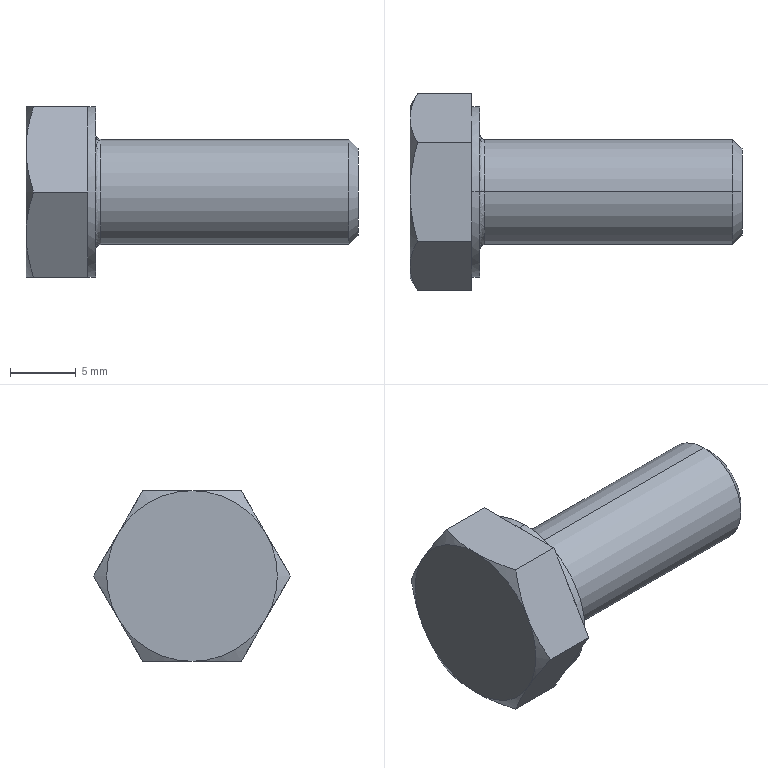Part | STEP file | Microwave Drying Flat Conveyor-hex screw gradeab_din_DIN EN 24017 - M8 x 20-N_Default | 1 solid | 29 faces | box 25.3 x 15.011 x 13 mm | volume 1766 mm3 | plane 15 | cone 8 | cylinder 4 | spline 2 | commonest cylinder face diameters 8 x2 13 x2
STEP:
#1=CARTESIAN_POINT('',(5.3,0.,4.4));
#2=VERTEX_POINT('',#1);
#3=CARTESIAN_POINT('',(5.3,0.,-4.4));
#4=VERTEX_POINT('',#3);
#5=CARTESIAN_POINT('',(5.3,0.,4.4));
#6=CARTESIAN_POINT('',(5.3,0.2797,4.4));
#7=CARTESIAN_POINT('',(5.3,0.6919,4.361));
#8=CARTESIAN_POINT('',(5.3,1.16,4.249));
#9=CARTESIAN_POINT('',(5.3,1.391,4.176));
#10=CARTESIAN_POINT('',(5.3,1.489,4.141));
#11=CARTESIAN_POINT('',(5.3,1.554,4.116));
#12=CARTESIAN_POINT('',(5.3,1.585,4.105));
#13=CARTESIAN_POINT('',(5.3,1.758,4.036));
#14=CARTESIAN_POINT('',(5.3,1.96,3.944));
#15=CARTESIAN_POINT('',(5.3,2.154,3.837));
#16=CARTESIAN_POINT('',(5.3,2.282,3.763));
#17=CARTESIAN_POINT('',(5.3,2.344,3.724));
#18=CARTESIAN_POINT('',(5.3,2.662,3.517));
#19=CARTESIAN_POINT('',(5.3,2.897,3.326));
#20=CARTESIAN_POINT('',(5.3,3.219,3.004));
#21=CARTESIAN_POINT('',(5.3,3.37,2.836));
#22=CARTESIAN_POINT('',(5.3,3.509,2.656));
#23=CARTESIAN_POINT('',(5.3,3.598,2.534));
#24=CARTESIAN_POINT('',(5.3,3.642,2.47));
#25=CARTESIAN_POINT('',(5.3,3.764,2.283));
#26=CARTESIAN_POINT('',(5.3,3.876,2.092));
#27=CARTESIAN_POINT('',(5.3,3.989,1.859));
#28=CARTESIAN_POINT('',(5.3,4.042,1.74));
#29=CARTESIAN_POINT('',(5.3,4.063,1.689));
#30=CARTESIAN_POINT('',(5.3,4.077,1.654));
#31=CARTESIAN_POINT('',(5.3,4.085,1.636));
#32=CARTESIAN_POINT('',(5.3,4.297,1.1));
#33=CARTESIAN_POINT('',(5.3,4.4,0.5592));
#34=CARTESIAN_POINT('',(5.3,4.4,-0.2796));
#35=CARTESIAN_POINT('',(5.3,4.361,-0.6917));
#36=CARTESIAN_POINT('',(5.3,4.249,-1.16));
#37=CARTESIAN_POINT('',(5.3,4.176,-1.391));
#38=CARTESIAN_POINT('',(5.3,4.141,-1.489));
#39=CARTESIAN_POINT('',(5.3,4.116,-1.554));
#40=CARTESIAN_POINT('',(5.3,4.105,-1.585));
#41=CARTESIAN_POINT('',(5.3,4.036,-1.758));
#42=CARTESIAN_POINT('',(5.3,3.944,-1.96));
#43=CARTESIAN_POINT('',(5.3,3.837,-2.154));
#44=CARTESIAN_POINT('',(5.3,3.763,-2.282));
#45=CARTESIAN_POINT('',(5.3,3.724,-2.344));
#46=CARTESIAN_POINT('',(5.3,3.517,-2.662));
#47=CARTESIAN_POINT('',(5.3,3.326,-2.897));
#48=CARTESIAN_POINT('',(5.3,3.004,-3.219));
#49=CARTESIAN_POINT('',(5.3,2.836,-3.37));
#50=CARTESIAN_POINT('',(5.3,2.656,-3.509));
#51=CARTESIAN_POINT('',(5.3,2.534,-3.598));
#52=CARTESIAN_POINT('',(5.3,2.47,-3.642));
#53=CARTESIAN_POINT('',(5.3,2.283,-3.764));
#54=CARTESIAN_POINT('',(5.3,2.092,-3.876));
#55=CARTESIAN_POINT('',(5.3,1.859,-3.989));
#56=CARTESIAN_POINT('',(5.3,1.74,-4.042));
#57=CARTESIAN_POINT('',(5.3,1.689,-4.063));
#58=CARTESIAN_POINT('',(5.3,1.654,-4.077));
#59=CARTESIAN_POINT('',(5.3,1.636,-4.085));
#60=CARTESIAN_POINT('',(5.3,1.1,-4.297));
#61=CARTESIAN_POINT('',(5.3,0.5597,-4.4));
#62=CARTESIAN_POINT('',(5.3,0.,-4.4));
#63=B_SPLINE_CURVE_WITH_KNOTS('',3,(#5,#6,#7,#8,#9,#10,#11,#12,#13,#14,#15,#16,#17,#18,#19,#20,#21,#22,#23,#24,#25,#26,#27,#28,#29,#30,#31,#32,#33,#34,#35,#36,#37,#38,#39,#40,#41,#42,#43,#44,#45,#46,#47,#48,#49,#50,#51,#52,#53,#54,#55,#56,#57,#58,#59,#60,#61,#62),.UNSPECIFIED.,.F.,.F.,(4,1,1,1,2,2,1,2,2,2,1,2,2,1,1,1,2,2,2,1,1,1,2,2,1,2,2,2,1,2,2,1,1,1,2,2,4),(0.,0.0625,0.09375,0.1094,0.1172,0.125,0.1562,0.1719,0.1875,0.25,0.2812,0.2969,0.3125,0.3437,0.3594,0.3672,0.3711,0.375,0.5,0.5625,0.5937,0.6094,0.6172,0.625,0.6562,0.6719,0.6875,0.75,0.7812,0.7969,0.8125,0.8437,0.8594,0.8672,0.8711,0.875,1.),.UNSPECIFIED.);
#64=EDGE_CURVE('',#2,#4,#63,.T.);
#65=ORIENTED_EDGE('',*,*,#64,.F.);
#66=CARTESIAN_POINT('',(5.7,0.,4.));
#67=VERTEX_POINT('',#66);
#68=CARTESIAN_POINT('',(5.7,0.,4.4));
#69=DIRECTION('',(0.,-1.,0.));
#70=DIRECTION('',(0.,0.,1.));
#71=AXIS2_PLACEMENT_3D('',#68,#69,#70);
#72=CIRCLE('',#71,0.4);
#73=EDGE_CURVE('',#2,#67,#72,.T.);
#74=ORIENTED_EDGE('',*,*,#73,.T.);
#75=CARTESIAN_POINT('',(5.7,0.,-4.));
#76=VERTEX_POINT('',#75);
#77=CARTESIAN_POINT('',(5.7,0.,0.));
#78=DIRECTION('',(1.,0.,0.));
#79=DIRECTION('',(0.,0.,1.));
#80=AXIS2_PLACEMENT_3D('',#77,#78,#79);
#81=CIRCLE('',#80,4.);
#82=EDGE_CURVE('',#76,#67,#81,.T.);
#83=ORIENTED_EDGE('',*,*,#82,.F.);
#84=CARTESIAN_POINT('',(5.7,0.,-4.4));
#85=DIRECTION('',(0.,1.,0.));
#86=DIRECTION('',(0.,0.,-1.));
#87=AXIS2_PLACEMENT_3D('',#84,#85,#86);
#88=CIRCLE('',#87,0.4);
#89=EDGE_CURVE('',#4,#76,#88,.T.);
#90=ORIENTED_EDGE('',*,*,#89,.F.);
#91=EDGE_LOOP('',(#65,#74,#83,#90));
#92=FACE_OUTER_BOUND('',#91,.T.);
#93=CARTESIAN_POINT('',(5.3,0.,-4.4));
#94=CARTESIAN_POINT('',(5.3,8.8,-4.4));
#95=CARTESIAN_POINT('',(5.3,8.8,4.4));
#96=CARTESIAN_POINT('',(5.3,0.,4.4));
#97=CARTESIAN_POINT('',(5.3,0.,-4.166));
#98=CARTESIAN_POINT('',(5.3,8.331,-4.166));
#99=CARTESIAN_POINT('',(5.3,8.331,4.166));
#100=CARTESIAN_POINT('',(5.3,0.,4.166));
#101=CARTESIAN_POINT('',(5.466,0.,-4.));
#102=CARTESIAN_POINT('',(5.466,8.,-4.));
#103=CARTESIAN_POINT('',(5.466,8.,4.));
#104=CARTESIAN_POINT('',(5.466,0.,4.));
#105=CARTESIAN_POINT('',(5.7,0.,-4.));
#106=CARTESIAN_POINT('',(5.7,8.,-4.));
#107=CARTESIAN_POINT('',(5.7,8.,4.));
#108=CARTESIAN_POINT('',(5.7,0.,4.));
#109=(BOUNDED_SURFACE()B_SPLINE_SURFACE(3,3,((#93,#94,#95,#96),(#97,#98,#99,#100),(#101,#102,#103,#104),(#105,#106,#107,#108)),.UNSPECIFIED.,.F.,.F.,.T.)B_SPLINE_SURFACE_WITH_KNOTS((4,4),(4,4),(0.,1.),(0.,1.),.UNSPECIFIED.)GEOMETRIC_REPRESENTATION_ITEM()RATIONAL_B_SPLINE_SURFACE(((1.,0.3333,0.3333,1.),(0.8047,0.2682,0.2682,0.8047),(0.8047,0.2682,0.2682,0.8047),(1.,0.3333,0.3333,1.)))REPRESENTATION_ITEM('')SURFACE());
#110=ADVANCED_FACE('',(#92),#109,.F.);
#111=CARTESIAN_POINT('',(24.609,0.,4.));
#112=VERTEX_POINT('',#111);
#113=CARTESIAN_POINT('',(24.609,0.,-4.));
#114=VERTEX_POINT('',#113);
#115=CARTESIAN_POINT('',(24.609,0.,0.));
#116=DIRECTION('',(-1.,0.,0.));
#117=DIRECTION('',(0.,0.,1.));
#118=AXIS2_PLACEMENT_3D('',#115,#116,#117);
#119=CIRCLE('',#118,4.);
#120=EDGE_CURVE('',#112,#114,#119,.T.);
#121=ORIENTED_EDGE('',*,*,#120,.T.);
#122=CARTESIAN_POINT('',(0.,0.,-4.));
#123=DIRECTION('',(-1.,0.,0.));
#124=VECTOR('',#123,1000.);
#125=LINE('',#122,#124);
#126=EDGE_CURVE('',#114,#76,#125,.T.);
#127=ORIENTED_EDGE('',*,*,#126,.T.);
#128=ORIENTED_EDGE('',*,*,#82,.T.);
#129=CARTESIAN_POINT('',(0.,0.,4.));
#130=DIRECTION('',(-1.,0.,0.));
#131=VECTOR('',#130,1000.);
#132=LINE('',#129,#131);
#133=EDGE_CURVE('',#112,#67,#132,.T.);
#134=ORIENTED_EDGE('',*,*,#133,.F.);
#135=EDGE_LOOP('',(#121,#127,#128,#134));
#136=FACE_OUTER_BOUND('',#135,.T.);
#137=CARTESIAN_POINT('',(0.,0.,0.));
#138=DIRECTION('',(-1.,0.,0.));
#139=DIRECTION('',(0.,0.,1.));
#140=AXIS2_PLACEMENT_3D('',#137,#138,#139);
#141=CYLINDRICAL_SURFACE('',#140,4.);
#142=ADVANCED_FACE('',(#136),#141,.T.);
#143=CARTESIAN_POINT('',(25.3,0.,3.31));
#144=VERTEX_POINT('',#143);
#145=CARTESIAN_POINT('',(25.3,0.,-3.31));
#146=VERTEX_POINT('',#145);
#147=CARTESIAN_POINT('',(25.3,0.,0.));
#148=DIRECTION('',(-1.,0.,0.));
#149=DIRECTION('',(0.,0.,1.));
#150=AXIS2_PLACEMENT_3D('',#147,#148,#149);
#151=CIRCLE('',#150,3.31);
#152=EDGE_CURVE('',#144,#146,#151,.T.);
#153=ORIENTED_EDGE('',*,*,#152,.T.);
#154=CARTESIAN_POINT('',(24.61,0.,-4.));
#155=DIRECTION('',(-0.7071,0.,-0.7071));
#156=VECTOR('',#155,1000.);
#157=LINE('',#154,#156);
#158=EDGE_CURVE('',#146,#114,#157,.T.);
#159=ORIENTED_EDGE('',*,*,#158,.T.);
#160=ORIENTED_EDGE('',*,*,#120,.F.);
#161=CARTESIAN_POINT('',(24.61,0.,4.));
#162=DIRECTION('',(-0.7071,0.,0.7071));
#163=VECTOR('',#162,1000.);
#164=LINE('',#161,#163);
#165=EDGE_CURVE('',#144,#112,#164,.T.);
#166=ORIENTED_EDGE('',*,*,#165,.F.);
#167=EDGE_LOOP('',(#153,#159,#160,#166));
#168=FACE_OUTER_BOUND('',#167,.T.);
#169=CARTESIAN_POINT('',(24.61,0.,0.));
#170=DIRECTION('',(-1.,0.,0.));
#171=DIRECTION('',(0.,0.,1.));
#172=AXIS2_PLACEMENT_3D('',#169,#170,#171);
#173=CONICAL_SURFACE('',#172,4.,0.7854);
#174=ADVANCED_FACE('',(#168),#173,.T.);
#175=CARTESIAN_POINT('',(5.3,0.,-6.5));
#176=VERTEX_POINT('',#175);
#177=CARTESIAN_POINT('',(5.3,0.,6.5));
#178=VERTEX_POINT('',#177);
#179=CARTESIAN_POINT('',(5.3,0.,0.));
#180=DIRECTION('',(1.,0.,0.));
#181=DIRECTION('',(0.,0.,1.));
#182=AXIS2_PLACEMENT_3D('',#179,#180,#181);
#183=CIRCLE('',#182,6.5);
#184=EDGE_CURVE('',#176,#178,#183,.T.);
#185=ORIENTED_EDGE('',*,*,#184,.F.);
#186=CARTESIAN_POINT('',(4.7,0.,-6.5));
#187=VERTEX_POINT('',#186);
#188=CARTESIAN_POINT('',(0.,0.,-6.5));
#189=DIRECTION('',(-1.,0.,0.));
#190=VECTOR('',#189,1000.);
#191=LINE('',#188,#190);
#192=EDGE_CURVE('',#176,#187,#191,.T.);
#193=ORIENTED_EDGE('',*,*,#192,.T.);
#194=CARTESIAN_POINT('',(4.7,5.629,-3.25));
#195=VERTEX_POINT('',#194);
#196=CARTESIAN_POINT('',(4.7,0.,0.));
#197=DIRECTION('',(1.,0.,0.));
#198=DIRECTION('',(0.,0.,1.));
#199=AXIS2_PLACEMENT_3D('',#196,#197,#198);
#200=CIRCLE('',#199,6.5);
#201=EDGE_CURVE('',#187,#195,#200,.T.);
#202=ORIENTED_EDGE('',*,*,#201,.T.);
#203=CARTESIAN_POINT('',(4.7,5.629,3.25));
#204=VERTEX_POINT('',#203);
#205=CARTESIAN_POINT('',(4.7,0.,0.));
#206=DIRECTION('',(1.,0.,0.));
#207=DIRECTION('',(0.,0.,1.));
#208=AXIS2_PLACEMENT_3D('',#205,#206,#207);
#209=CIRCLE('',#208,6.5);
#210=EDGE_CURVE('',#195,#204,#209,.T.);
#211=ORIENTED_EDGE('',*,*,#210,.T.);
#212=CARTESIAN_POINT('',(4.7,0.,6.5));
#213=VERTEX_POINT('',#212);
#214=CARTESIAN_POINT('',(4.7,0.,0.));
#215=DIRECTION('',(1.,0.,0.));
#216=DIRECTION('',(0.,0.,1.));
#217=AXIS2_PLACEMENT_3D('',#214,#215,#216);
#218=CIRCLE('',#217,6.5);
#219=EDGE_CURVE('',#204,#213,#218,.T.);
#220=ORIENTED_EDGE('',*,*,#219,.T.);
#221=CARTESIAN_POINT('',(0.,0.,6.5));
#222=DIRECTION('',(-1.,0.,0.));
#223=VECTOR('',#222,1000.);
#224=LINE('',#221,#223);
#225=EDGE_CURVE('',#178,#213,#224,.T.);
#226=ORIENTED_EDGE('',*,*,#225,.F.);
#227=EDGE_LOOP('',(#185,#193,#202,#211,#220,#226));
#228=FACE_OUTER_BOUND('',#227,.T.);
#229=CARTESIAN_POINT('',(0.,0.,0.));
#230=DIRECTION('',(-1.,0.,0.));
#231=DIRECTION('',(0.,0.,1.));
#232=AXIS2_PLACEMENT_3D('',#229,#230,#231);
#233=CYLINDRICAL_SURFACE('',#232,6.5);
#234=ADVANCED_FACE('',(#228),#233,.T.);
#235=ORIENTED_EDGE('',*,*,#126,.F.);
#236=CARTESIAN_POINT('',(24.609,0.,0.));
#237=DIRECTION('',(-1.,0.,0.));
#238=DIRECTION('',(0.,0.,1.));
#239=AXIS2_PLACEMENT_3D('',#236,#237,#238);
#240=CIRCLE('',#239,4.);
#241=EDGE_CURVE('',#114,#112,#240,.T.);
#242=ORIENTED_EDGE('',*,*,#241,.T.);
#243=ORIENTED_EDGE('',*,*,#133,.T.);
#244=CARTESIAN_POINT('',(5.7,0.,0.));
#245=DIRECTION('',(1.,0.,0.));
#246=DIRECTION('',(0.,0.,1.));
#247=AXIS2_PLACEMENT_3D('',#244,#245,#246);
#248=CIRCLE('',#247,4.);
#249=EDGE_CURVE('',#67,#76,#248,.T.);
#250=ORIENTED_EDGE('',*,*,#249,.T.);
#251=EDGE_LOOP('',(#235,#242,#243,#250));
#252=FACE_OUTER_BOUND('',#251,.T.);
#253=CARTESIAN_POINT('',(0.,0.,0.));
#254=DIRECTION('',(-1.,0.,0.));
#255=DIRECTION('',(0.,0.,1.));
#256=AXIS2_PLACEMENT_3D('',#253,#254,#255);
#257=CYLINDRICAL_SURFACE('',#256,4.);
#258=ADVANCED_FACE('',(#252),#257,.T.);
#259=ORIENTED_EDGE('',*,*,#73,.F.);
#260=CARTESIAN_POINT('',(5.3,0.,-4.4));
#261=CARTESIAN_POINT('',(5.3,-0.2797,-4.4));
#262=CARTESIAN_POINT('',(5.3,-0.6919,-4.361));
#263=CARTESIAN_POINT('',(5.3,-1.16,-4.249));
#264=CARTESIAN_POINT('',(5.3,-1.391,-4.176));
#265=CARTESIAN_POINT('',(5.3,-1.489,-4.141));
#266=CARTESIAN_POINT('',(5.3,-1.554,-4.116));
#267=CARTESIAN_POINT('',(5.3,-1.585,-4.105));
#268=CARTESIAN_POINT('',(5.3,-1.758,-4.036));
#269=CARTESIAN_POINT('',(5.3,-1.96,-3.944));
#270=CARTESIAN_POINT('',(5.3,-2.154,-3.837));
#271=CARTESIAN_POINT('',(5.3,-2.282,-3.763));
#272=CARTESIAN_POINT('',(5.3,-2.344,-3.724));
#273=CARTESIAN_POINT('',(5.3,-2.662,-3.517));
#274=CARTESIAN_POINT('',(5.3,-2.897,-3.326));
#275=CARTESIAN_POINT('',(5.3,-3.219,-3.004));
#276=CARTESIAN_POINT('',(5.3,-3.37,-2.836));
#277=CARTESIAN_POINT('',(5.3,-3.509,-2.656));
#278=CARTESIAN_POINT('',(5.3,-3.598,-2.534));
#279=CARTESIAN_POINT('',(5.3,-3.642,-2.47));
#280=CARTESIAN_POINT('',(5.3,-3.764,-2.283));
#281=CARTESIAN_POINT('',(5.3,-3.876,-2.092));
#282=CARTESIAN_POINT('',(5.3,-3.989,-1.859));
#283=CARTESIAN_POINT('',(5.3,-4.042,-1.74));
#284=CARTESIAN_POINT('',(5.3,-4.063,-1.689));
#285=CARTESIAN_POINT('',(5.3,-4.077,-1.654));
#286=CARTESIAN_POINT('',(5.3,-4.085,-1.636));
#287=CARTESIAN_POINT('',(5.3,-4.297,-1.1));
#288=CARTESIAN_POINT('',(5.3,-4.4,-0.5592));
#289=CARTESIAN_POINT('',(5.3,-4.4,0.2796));
#290=CARTESIAN_POINT('',(5.3,-4.361,0.6917));
#291=CARTESIAN_POINT('',(5.3,-4.249,1.16));
#292=CARTESIAN_POINT('',(5.3,-4.176,1.391));
#293=CARTESIAN_POINT('',(5.3,-4.141,1.489));
#294=CARTESIAN_POINT('',(5.3,-4.116,1.554));
#295=CARTESIAN_POINT('',(5.3,-4.105,1.585));
#296=CARTESIAN_POINT('',(5.3,-4.036,1.758));
#297=CARTESIAN_POINT('',(5.3,-3.944,1.96));
#298=CARTESIAN_POINT('',(5.3,-3.837,2.154));
#299=CARTESIAN_POINT('',(5.3,-3.763,2.282));
#300=CARTESIAN_POINT('',(5.3,-3.724,2.344));
#301=CARTESIAN_POINT('',(5.3,-3.517,2.662));
#302=CARTESIAN_POINT('',(5.3,-3.326,2.897));
#303=CARTESIAN_POINT('',(5.3,-3.004,3.219));
#304=CARTESIAN_POINT('',(5.3,-2.836,3.37));
#305=CARTESIAN_POINT('',(5.3,-2.656,3.509));
#306=CARTESIAN_POINT('',(5.3,-2.534,3.598));
#307=CARTESIAN_POINT('',(5.3,-2.47,3.642));
#308=CARTESIAN_POINT('',(5.3,-2.283,3.764));
#309=CARTESIAN_POINT('',(5.3,-2.092,3.876));
#310=CARTESIAN_POINT('',(5.3,-1.859,3.989));
#311=CARTESIAN_POINT('',(5.3,-1.74,4.042));
#312=CARTESIAN_POINT('',(5.3,-1.689,4.063));
#313=CARTESIAN_POINT('',(5.3,-1.654,4.077));
#314=CARTESIAN_POINT('',(5.3,-1.636,4.085));
#315=CARTESIAN_POINT('',(5.3,-1.1,4.297));
#316=CARTESIAN_POINT('',(5.3,-0.5597,4.4));
#317=CARTESIAN_POINT('',(5.3,0.,4.4));
#318=B_SPLINE_CURVE_WITH_KNOTS('',3,(#260,#261,#262,#263,#264,#265,#266,#267,#268,#269,#270,#271,#272,#273,#274,#275,#276,#277,#278,#279,#280,#281,#282,#283,#284,#285,#286,#287,#288,#289,#290,#291,#292,#293,#294,#295,#296,#297,#298,#299,#300,#301,#302,#303,#304,#305,#306,#307,#308,#309,#310,#311,#312,#313,#314,#315,#316,#317),.UNSPECIFIED.,.F.,.F.,(4,1,1,1,2,2,1,2,2,2,1,2,2,1,1,1,2,2,2,1,1,1,2,2,1,2,2,2,1,2,2,1,1,1,2,2,4),(0.,0.0625,0.09375,0.1094,0.1172,0.125,0.1563,0.1719,0.1875,0.25,0.2812,0.2969,0.3125,0.3437,0.3594,0.3672,0.3711,0.375,0.5,0.5625,0.5937,0.6094,0.6172,0.625,0.6563,0.6719,0.6875,0.75,0.7813,0.7969,0.8125,0.8438,0.8594,0.8672,0.8711,0.875,1.),.UNSPECIFIED.);
#319=EDGE_CURVE('',#4,#2,#318,.T.);
#320=ORIENTED_EDGE('',*,*,#319,.F.);
#321=ORIENTED_EDGE('',*,*,#89,.T.);
#322=ORIENTED_EDGE('',*,*,#249,.F.);
#323=EDGE_LOOP('',(#259,#320,#321,#322));
#324=FACE_OUTER_BOUND('',#323,.T.);
#325=CARTESIAN_POINT('',(5.3,0.,4.4));
#326=CARTESIAN_POINT('',(5.3,-8.8,4.4));
#327=CARTESIAN_POINT('',(5.3,-8.8,-4.4));
#328=CARTESIAN_POINT('',(5.3,0.,-4.4));
#329=CARTESIAN_POINT('',(5.3,0.,4.166));
#330=CARTESIAN_POINT('',(5.3,-8.331,4.166));
#331=CARTESIAN_POINT('',(5.3,-8.331,-4.166));
#332=CARTESIAN_POINT('',(5.3,0.,-4.166));
#333=CARTESIAN_POINT('',(5.466,0.,4.));
#334=CARTESIAN_POINT('',(5.466,-8.,4.));
#335=CARTESIAN_POINT('',(5.466,-8.,-4.));
#336=CARTESIAN_POINT('',(5.466,0.,-4.));
#337=CARTESIAN_POINT('',(5.7,0.,4.));
#338=CARTESIAN_POINT('',(5.7,-8.,4.));
#339=CARTESIAN_POINT('',(5.7,-8.,-4.));
#340=CARTESIAN_POINT('',(5.7,0.,-4.));
#341=(BOUNDED_SURFACE()B_SPLINE_SURFACE(3,3,((#325,#326,#327,#328),(#329,#330,#331,#332),(#333,#334,#335,#336),(#337,#338,#339,#340)),.UNSPECIFIED.,.F.,.F.,.F.)B_SPLINE_SURFACE_WITH_KNOTS((4,4),(4,4),(0.,1.),(0.,1.),.UNSPECIFIED.)GEOMETRIC_REPRESENTATION_ITEM()RATIONAL_B_SPLINE_SURFACE(((1.,0.3333,0.3333,1.),(0.8047,0.2682,0.2682,0.8047),(0.8047,0.2682,0.2682,0.8047),(1.,0.3333,0.3333,1.)))REPRESENTATION_ITEM('')SURFACE());
#342=ADVANCED_FACE('',(#324),#341,.F.);
#343=ORIENTED_EDGE('',*,*,#158,.F.);
#344=CARTESIAN_POINT('',(25.3,0.,0.));
#345=DIRECTION('',(-1.,0.,0.));
#346=DIRECTION('',(0.,0.,1.));
#347=AXIS2_PLACEMENT_3D('',#344,#345,#346);
#348=CIRCLE('',#347,3.31);
#349=EDGE_CURVE('',#146,#144,#348,.T.);
#350=ORIENTED_EDGE('',*,*,#349,.T.);
#351=ORIENTED_EDGE('',*,*,#165,.T.);
#352=ORIENTED_EDGE('',*,*,#241,.F.);
#353=EDGE_LOOP('',(#343,#350,#351,#352));
#354=FACE_OUTER_BOUND('',#353,.T.);
#355=CARTESIAN_POINT('',(24.61,0.,0.));
#356=DIRECTION('',(-1.,0.,0.));
#357=DIRECTION('',(0.,0.,1.));
#358=AXIS2_PLACEMENT_3D('',#355,#356,#357);
#359=CONICAL_SURFACE('',#358,4.,0.7854);
#360=ADVANCED_FACE('',(#354),#359,.T.);
#361=CARTESIAN_POINT('',(5.3,0.,0.));
#362=DIRECTION('',(1.,0.,0.));
#363=DIRECTION('',(0.,0.,1.));
#364=AXIS2_PLACEMENT_3D('',#361,#362,#363);
#365=CIRCLE('',#364,6.5);
#366=EDGE_CURVE('',#178,#176,#365,.T.);
#367=ORIENTED_EDGE('',*,*,#366,.T.);
#368=ORIENTED_EDGE('',*,*,#184,.T.);
#369=EDGE_LOOP('',(#367,#368));
#370=FACE_OUTER_BOUND('',#369,.T.);
#371=ORIENTED_EDGE('',*,*,#319,.T.);
#372=ORIENTED_EDGE('',*,*,#64,.T.);
#373=EDGE_LOOP('',(#371,#372));
#374=FACE_BOUND('',#373,.T.);
#375=CARTESIAN_POINT('',(5.3,7.506,0.));
#376=DIRECTION('',(1.,0.,0.));
#377=DIRECTION('',(0.,0.,-1.));
#378=AXIS2_PLACEMENT_3D('',#375,#376,#377);
#379=PLANE('',#378);
#380=ADVANCED_FACE('',(#370,#374),#379,.T.);
#381=ORIENTED_EDGE('',*,*,#152,.F.);
#382=ORIENTED_EDGE('',*,*,#349,.F.);
#383=EDGE_LOOP('',(#381,#382));
#384=FACE_OUTER_BOUND('',#383,.T.);
#385=CARTESIAN_POINT('',(25.3,0.,0.));
#386=DIRECTION('',(-1.,0.,0.));
#387=DIRECTION('',(0.,0.,1.));
#388=AXIS2_PLACEMENT_3D('',#385,#386,#387);
#389=PLANE('',#388);
#390=ADVANCED_FACE('',(#384),#389,.F.);
#391=ORIENTED_EDGE('',*,*,#192,.F.);
#392=ORIENTED_EDGE('',*,*,#366,.F.);
#393=ORIENTED_EDGE('',*,*,#225,.T.);
#394=CARTESIAN_POINT('',(4.7,-5.629,3.25));
#395=VERTEX_POINT('',#394);
#396=CARTESIAN_POINT('',(4.7,0.,0.));
#397=DIRECTION('',(1.,0.,0.));
#398=DIRECTION('',(0.,0.,1.));
#399=AXIS2_PLACEMENT_3D('',#396,#397,#398);
#400=CIRCLE('',#399,6.5);
#401=EDGE_CURVE('',#213,#395,#400,.T.);
#402=ORIENTED_EDGE('',*,*,#401,.T.);
#403=CARTESIAN_POINT('',(4.7,-5.629,-3.25));
#404=VERTEX_POINT('',#403);
#405=CARTESIAN_POINT('',(4.7,0.,0.));
#406=DIRECTION('',(1.,0.,0.));
#407=DIRECTION('',(0.,0.,1.));
#408=AXIS2_PLACEMENT_3D('',#405,#406,#407);
#409=CIRCLE('',#408,6.5);
#410=EDGE_CURVE('',#395,#404,#409,.T.);
#411=ORIENTED_EDGE('',*,*,#410,.T.);
#412=CARTESIAN_POINT('',(4.7,0.,0.));
#413=DIRECTION('',(1.,0.,0.));
#414=DIRECTION('',(0.,0.,1.));
#415=AXIS2_PLACEMENT_3D('',#412,#413,#414);
#416=CIRCLE('',#415,6.5);
#417=EDGE_CURVE('',#404,#187,#416,.T.);
#418=ORIENTED_EDGE('',*,*,#417,.T.);
#419=EDGE_LOOP('',(#391,#392,#393,#402,#411,#418));
#420=FACE_OUTER_BOUND('',#419,.T.);
#421=CARTESIAN_POINT('',(0.,0.,0.));
#422=DIRECTION('',(-1.,0.,0.));
#423=DIRECTION('',(0.,0.,1.));
#424=AXIS2_PLACEMENT_3D('',#421,#422,#423);
#425=CYLINDRICAL_SURFACE('',#424,6.5);
#426=ADVANCED_FACE('',(#420),#425,.T.);
#427=CARTESIAN_POINT('',(4.7,3.753,6.5));
#428=VERTEX_POINT('',#427);
#429=CARTESIAN_POINT('',(4.7,6.5,6.5));
#430=DIRECTION('',(0.,-1.,0.));
#431=VECTOR('',#430,1000.);
#432=LINE('',#429,#431);
#433=EDGE_CURVE('',#428,#213,#432,.T.);
#434=ORIENTED_EDGE('',*,*,#433,.T.);
#435=ORIENTED_EDGE('',*,*,#219,.F.);
#436=CARTESIAN_POINT('',(4.7,5.629,3.25));
#437=DIRECTION('',(0.,-0.5,0.866));
#438=VECTOR('',#437,1000.);
#439=LINE('',#436,#438);
#440=EDGE_CURVE('',#204,#428,#439,.T.);
#441=ORIENTED_EDGE('',*,*,#440,.T.);
#442=EDGE_LOOP('',(#434,#435,#441));
#443=FACE_OUTER_BOUND('',#442,.T.);
#444=CARTESIAN_POINT('',(4.7,6.5,0.));
#445=DIRECTION('',(1.,0.,0.));
#446=DIRECTION('',(0.,0.,-1.));
#447=AXIS2_PLACEMENT_3D('',#444,#445,#446);
#448=PLANE('',#447);
#449=ADVANCED_FACE('',(#443),#448,.T.);
#450=CARTESIAN_POINT('',(4.7,7.506,0.));
#451=VERTEX_POINT('',#450);
#452=CARTESIAN_POINT('',(4.7,7.506,0.));
#453=DIRECTION('',(0.,-0.5,0.866));
#454=VECTOR('',#453,1000.);
#455=LINE('',#452,#454);
#456=EDGE_CURVE('',#451,#204,#455,.T.);
#457=ORIENTED_EDGE('',*,*,#456,.T.);
#458=ORIENTED_EDGE('',*,*,#210,.F.);
#459=CARTESIAN_POINT('',(4.7,5.629,-3.25));
#460=DIRECTION('',(0.,0.5,0.866));
#461=VECTOR('',#460,1000.);
#462=LINE('',#459,#461);
#463=EDGE_CURVE('',#195,#451,#462,.T.);
#464=ORIENTED_EDGE('',*,*,#463,.T.);
#465=EDGE_LOOP('',(#457,#458,#464));
#466=FACE_OUTER_BOUND('',#465,.T.);
#467=CARTESIAN_POINT('',(4.7,6.5,0.));
#468=DIRECTION('',(1.,0.,0.));
#469=DIRECTION('',(0.,0.,-1.));
#470=AXIS2_PLACEMENT_3D('',#467,#468,#469);
#471=PLANE('',#470);
#472=ADVANCED_FACE('',(#466),#471,.T.);
#473=ORIENTED_EDGE('',*,*,#201,.F.);
#474=CARTESIAN_POINT('',(4.7,3.753,-6.5));
#475=VERTEX_POINT('',#474);
#476=CARTESIAN_POINT('',(4.7,6.5,-6.5));
#477=DIRECTION('',(0.,1.,0.));
#478=VECTOR('',#477,1000.);
#479=LINE('',#476,#478);
#480=EDGE_CURVE('',#187,#475,#479,.T.);
#481=ORIENTED_EDGE('',*,*,#480,.T.);
#482=CARTESIAN_POINT('',(4.7,3.753,-6.5));
#483=DIRECTION('',(0.,0.5,0.866));
#484=VECTOR('',#483,1000.);
#485=LINE('',#482,#484);
#486=EDGE_CURVE('',#475,#195,#485,.T.);
#487=ORIENTED_EDGE('',*,*,#486,.T.);
#488=EDGE_LOOP('',(#473,#481,#487));
#489=FACE_OUTER_BOUND('',#488,.T.);
#490=CARTESIAN_POINT('',(4.7,6.5,0.));
#491=DIRECTION('',(1.,0.,0.));
#492=DIRECTION('',(0.,0.,-1.));
#493=AXIS2_PLACEMENT_3D('',#490,#491,#492);
#494=PLANE('',#493);
#495=ADVANCED_FACE('',(#489),#494,.T.);
#496=CARTESIAN_POINT('',(4.7,-3.753,-6.5));
#497=VERTEX_POINT('',#496);
#498=CARTESIAN_POINT('',(4.7,6.5,-6.5));
#499=DIRECTION('',(0.,1.,0.));
#500=VECTOR('',#499,1000.);
#501=LINE('',#498,#500);
#502=EDGE_CURVE('',#497,#187,#501,.T.);
#503=ORIENTED_EDGE('',*,*,#502,.T.);
#504=ORIENTED_EDGE('',*,*,#417,.F.);
#505=CARTESIAN_POINT('',(4.7,-5.629,-3.25));
#506=DIRECTION('',(0.,0.5,-0.866));
#507=VECTOR('',#506,1000.);
#508=LINE('',#505,#507);
#509=EDGE_CURVE('',#404,#497,#508,.T.);
#510=ORIENTED_EDGE('',*,*,#509,.T.);
#511=EDGE_LOOP('',(#503,#504,#510));
#512=FACE_OUTER_BOUND('',#511,.T.);
#513=CARTESIAN_POINT('',(4.7,6.5,0.));
#514=DIRECTION('',(1.,0.,0.));
#515=DIRECTION('',(0.,0.,-1.));
#516=AXIS2_PLACEMENT_3D('',#513,#514,#515);
#517=PLANE('',#516);
#518=ADVANCED_FACE('',(#512),#517,.T.);
#519=CARTESIAN_POINT('',(4.7,-7.506,0.));
#520=VERTEX_POINT('',#519);
#521=CARTESIAN_POINT('',(4.7,-7.506,0.));
#522=DIRECTION('',(0.,0.5,-0.866));
#523=VECTOR('',#522,1000.);
#524=LINE('',#521,#523);
#525=EDGE_CURVE('',#520,#404,#524,.T.);
#526=ORIENTED_EDGE('',*,*,#525,.T.);
#527=ORIENTED_EDGE('',*,*,#410,.F.);
#528=CARTESIAN_POINT('',(4.7,-5.629,3.25));
#529=DIRECTION('',(0.,-0.5,-0.866));
#530=VECTOR('',#529,1000.);
#531=LINE('',#528,#530);
#532=EDGE_CURVE('',#395,#520,#531,.T.);
#533=ORIENTED_EDGE('',*,*,#532,.T.);
#534=EDGE_LOOP('',(#526,#527,#533));
#535=FACE_OUTER_BOUND('',#534,.T.);
#536=CARTESIAN_POINT('',(4.7,6.5,0.));
#537=DIRECTION('',(1.,0.,0.));
#538=DIRECTION('',(0.,0.,-1.));
#539=AXIS2_PLACEMENT_3D('',#536,#537,#538);
#540=PLANE('',#539);
#541=ADVANCED_FACE('',(#535),#540,.T.);
#542=CARTESIAN_POINT('',(4.7,-3.753,6.5));
#543=VERTEX_POINT('',#542);
#544=CARTESIAN_POINT('',(4.7,-3.753,6.5));
#545=DIRECTION('',(0.,-0.5,-0.866));
#546=VECTOR('',#545,1000.);
#547=LINE('',#544,#546);
#548=EDGE_CURVE('',#543,#395,#547,.T.);
#549=ORIENTED_EDGE('',*,*,#548,.T.);
#550=ORIENTED_EDGE('',*,*,#401,.F.);
#551=CARTESIAN_POINT('',(4.7,6.5,6.5));
#552=DIRECTION('',(0.,-1.,0.));
#553=VECTOR('',#552,1000.);
#554=LINE('',#551,#553);
#555=EDGE_CURVE('',#213,#543,#554,.T.);
#556=ORIENTED_EDGE('',*,*,#555,.T.);
#557=EDGE_LOOP('',(#549,#550,#556));
#558=FACE_OUTER_BOUND('',#557,.T.);
#559=CARTESIAN_POINT('',(4.7,6.5,0.));
#560=DIRECTION('',(1.,0.,0.));
#561=DIRECTION('',(0.,0.,-1.));
#562=AXIS2_PLACEMENT_3D('',#559,#560,#561);
#563=PLANE('',#562);
#564=ADVANCED_FACE('',(#558),#563,.T.);
#565=CARTESIAN_POINT('',(0.5806,3.753,6.5));
#566=VERTEX_POINT('',#565);
#567=CARTESIAN_POINT('',(5.3,3.753,6.5));
#568=DIRECTION('',(1.,0.,0.));
#569=VECTOR('',#568,1000.);
#570=LINE('',#567,#569);
#571=EDGE_CURVE('',#566,#428,#570,.T.);
#572=ORIENTED_EDGE('',*,*,#571,.F.);
#573=CARTESIAN_POINT('',(0.,0.,6.5));
#574=VERTEX_POINT('',#573);
#575=CARTESIAN_POINT('',(0.,0.,6.5));
#576=CARTESIAN_POINT('',(0.,1.281,6.5));
#577=CARTESIAN_POINT('',(0.2266,2.527,6.5));
#578=CARTESIAN_POINT('',(0.5806,3.753,6.5));
#579=B_SPLINE_CURVE_WITH_KNOTS('',3,(#575,#576,#577,#578),.UNSPECIFIED.,.F.,.F.,(4,4),(0.,0.003797),.UNSPECIFIED.);
#580=EDGE_CURVE('',#574,#566,#579,.T.);
#581=ORIENTED_EDGE('',*,*,#580,.F.);
#582=CARTESIAN_POINT('',(0.5806,-3.753,6.5));
#583=VERTEX_POINT('',#582);
#584=CARTESIAN_POINT('',(0.5806,-3.753,6.5));
#585=CARTESIAN_POINT('',(0.2266,-2.527,6.5));
#586=CARTESIAN_POINT('',(0.,-1.281,6.5));
#587=CARTESIAN_POINT('',(0.,0.,6.5));
#588=B_SPLINE_CURVE_WITH_KNOTS('',3,(#584,#585,#586,#587),.UNSPECIFIED.,.F.,.F.,(4,4),(0.,0.003797),.UNSPECIFIED.);
#589=EDGE_CURVE('',#583,#574,#588,.T.);
#590=ORIENTED_EDGE('',*,*,#589,.F.);
#591=CARTESIAN_POINT('',(5.3,-3.753,6.5));
#592=DIRECTION('',(-1.,0.,0.));
#593=VECTOR('',#592,1000.);
#594=LINE('',#591,#593);
#595=EDGE_CURVE('',#543,#583,#594,.T.);
#596=ORIENTED_EDGE('',*,*,#595,.F.);
#597=ORIENTED_EDGE('',*,*,#555,.F.);
#598=ORIENTED_EDGE('',*,*,#433,.F.);
#599=EDGE_LOOP('',(#572,#581,#590,#596,#597,#598));
#600=FACE_OUTER_BOUND('',#599,.T.);
#601=CARTESIAN_POINT('',(5.3,3.753,6.5));
#602=DIRECTION('',(0.,0.,-1.));
#603=DIRECTION('',(0.,1.,0.));
#604=AXIS2_PLACEMENT_3D('',#601,#602,#603);
#605=PLANE('',#604);
#606=ADVANCED_FACE('',(#600),#605,.F.);
#607=CARTESIAN_POINT('',(0.5806,7.506,0.));
#608=VERTEX_POINT('',#607);
#609=CARTESIAN_POINT('',(5.3,7.506,0.));
#610=DIRECTION('',(1.,0.,0.));
#611=VECTOR('',#610,1000.);
#612=LINE('',#609,#611);
#613=EDGE_CURVE('',#608,#451,#612,.T.);
#614=ORIENTED_EDGE('',*,*,#613,.F.);
#615=CARTESIAN_POINT('',(0.,5.629,3.25));
#616=VERTEX_POINT('',#615);
#617=CARTESIAN_POINT('',(0.,5.629,3.25));
#618=CARTESIAN_POINT('',(0.,6.27,2.141));
#619=CARTESIAN_POINT('',(0.2266,6.892,1.062));
#620=CARTESIAN_POINT('',(0.5806,7.506,0.));
#621=B_SPLINE_CURVE_WITH_KNOTS('',3,(#617,#618,#619,#620),.UNSPECIFIED.,.F.,.F.,(4,4),(0.,0.003797),.UNSPECIFIED.);
#622=EDGE_CURVE('',#616,#608,#621,.T.);
#623=ORIENTED_EDGE('',*,*,#622,.F.);
#624=CARTESIAN_POINT('',(0.5806,3.753,6.5));
#625=CARTESIAN_POINT('',(0.2266,4.366,5.438));
#626=CARTESIAN_POINT('',(0.,4.989,4.359));
#627=CARTESIAN_POINT('',(0.,5.629,3.25));
#628=B_SPLINE_CURVE_WITH_KNOTS('',3,(#624,#625,#626,#627),.UNSPECIFIED.,.F.,.F.,(4,4),(0.,0.003797),.UNSPECIFIED.);
#629=EDGE_CURVE('',#566,#616,#628,.T.);
#630=ORIENTED_EDGE('',*,*,#629,.F.);
#631=ORIENTED_EDGE('',*,*,#571,.T.);
#632=ORIENTED_EDGE('',*,*,#440,.F.);
#633=ORIENTED_EDGE('',*,*,#456,.F.);
#634=EDGE_LOOP('',(#614,#623,#630,#631,#632,#633));
#635=FACE_OUTER_BOUND('',#634,.T.);
#636=CARTESIAN_POINT('',(5.3,7.506,0.));
#637=DIRECTION('',(0.,-0.866,-0.5));
#638=DIRECTION('',(0.,0.5,-0.866));
#639=AXIS2_PLACEMENT_3D('',#636,#637,#638);
#640=PLANE('',#639);
#641=ADVANCED_FACE('',(#635),#640,.F.);
#642=CARTESIAN_POINT('',(0.5806,3.753,-6.5));
#643=VERTEX_POINT('',#642);
#644=CARTESIAN_POINT('',(5.3,3.753,-6.5));
#645=DIRECTION('',(1.,0.,0.));
#646=VECTOR('',#645,1000.);
#647=LINE('',#644,#646);
#648=EDGE_CURVE('',#643,#475,#647,.T.);
#649=ORIENTED_EDGE('',*,*,#648,.F.);
#650=CARTESIAN_POINT('',(0.,5.629,-3.25));
#651=VERTEX_POINT('',#650);
#652=CARTESIAN_POINT('',(0.,5.629,-3.25));
#653=CARTESIAN_POINT('',(0.,4.989,-4.359));
#654=CARTESIAN_POINT('',(0.2266,4.366,-5.438));
#655=CARTESIAN_POINT('',(0.5806,3.753,-6.5));
#656=B_SPLINE_CURVE_WITH_KNOTS('',3,(#652,#653,#654,#655),.UNSPECIFIED.,.F.,.F.,(4,4),(0.,0.003797),.UNSPECIFIED.);
#657=EDGE_CURVE('',#651,#643,#656,.T.);
#658=ORIENTED_EDGE('',*,*,#657,.F.);
#659=CARTESIAN_POINT('',(0.5806,7.506,0.));
#660=CARTESIAN_POINT('',(0.2266,6.892,-1.062));
#661=CARTESIAN_POINT('',(0.,6.27,-2.141));
#662=CARTESIAN_POINT('',(0.,5.629,-3.25));
#663=B_SPLINE_CURVE_WITH_KNOTS('',3,(#659,#660,#661,#662),.UNSPECIFIED.,.F.,.F.,(4,4),(0.,0.003797),.UNSPECIFIED.);
#664=EDGE_CURVE('',#608,#651,#663,.T.);
#665=ORIENTED_EDGE('',*,*,#664,.F.);
#666=ORIENTED_EDGE('',*,*,#613,.T.);
#667=ORIENTED_EDGE('',*,*,#463,.F.);
#668=ORIENTED_EDGE('',*,*,#486,.F.);
#669=EDGE_LOOP('',(#649,#658,#665,#666,#667,#668));
#670=FACE_OUTER_BOUND('',#669,.T.);
#671=CARTESIAN_POINT('',(5.3,3.753,-6.5));
#672=DIRECTION('',(0.,-0.866,0.5));
#673=DIRECTION('',(0.,-0.5,-0.866));
#674=AXIS2_PLACEMENT_3D('',#671,#672,#673);
#675=PLANE('',#674);
#676=ADVANCED_FACE('',(#670),#675,.F.);
#677=CARTESIAN_POINT('',(0.5806,-3.753,-6.5));
#678=VERTEX_POINT('',#677);
#679=CARTESIAN_POINT('',(5.3,-3.753,-6.5));
#680=DIRECTION('',(1.,0.,0.));
#681=VECTOR('',#680,1000.);
#682=LINE('',#679,#681);
#683=EDGE_CURVE('',#678,#497,#682,.T.);
#684=ORIENTED_EDGE('',*,*,#683,.F.);
#685=CARTESIAN_POINT('',(0.,0.,-6.5));
#686=VERTEX_POINT('',#685);
#687=CARTESIAN_POINT('',(0.,0.,-6.5));
#688=CARTESIAN_POINT('',(0.,-1.281,-6.5));
#689=CARTESIAN_POINT('',(0.2266,-2.527,-6.5));
#690=CARTESIAN_POINT('',(0.5806,-3.753,-6.5));
#691=B_SPLINE_CURVE_WITH_KNOTS('',3,(#687,#688,#689,#690),.UNSPECIFIED.,.F.,.F.,(4,4),(0.,0.003797),.UNSPECIFIED.);
#692=EDGE_CURVE('',#686,#678,#691,.T.);
#693=ORIENTED_EDGE('',*,*,#692,.F.);
#694=CARTESIAN_POINT('',(0.5806,3.753,-6.5));
#695=CARTESIAN_POINT('',(0.2266,2.527,-6.5));
#696=CARTESIAN_POINT('',(0.,1.281,-6.5));
#697=CARTESIAN_POINT('',(0.,0.,-6.5));
#698=B_SPLINE_CURVE_WITH_KNOTS('',3,(#694,#695,#696,#697),.UNSPECIFIED.,.F.,.F.,(4,4),(0.,0.003797),.UNSPECIFIED.);
#699=EDGE_CURVE('',#643,#686,#698,.T.);
#700=ORIENTED_EDGE('',*,*,#699,.F.);
#701=ORIENTED_EDGE('',*,*,#648,.T.);
#702=ORIENTED_EDGE('',*,*,#480,.F.);
#703=ORIENTED_EDGE('',*,*,#502,.F.);
#704=EDGE_LOOP('',(#684,#693,#700,#701,#702,#703));
#705=FACE_OUTER_BOUND('',#704,.T.);
#706=CARTESIAN_POINT('',(5.3,3.753,-6.5));
#707=DIRECTION('',(0.,0.,1.));
#708=DIRECTION('',(0.,-1.,0.));
#709=AXIS2_PLACEMENT_3D('',#706,#707,#708);
#710=PLANE('',#709);
#711=ADVANCED_FACE('',(#705),#710,.F.);
#712=CARTESIAN_POINT('',(0.5806,-7.506,0.));
#713=VERTEX_POINT('',#712);
#714=CARTESIAN_POINT('',(5.3,-7.506,0.));
#715=DIRECTION('',(1.,0.,0.));
#716=VECTOR('',#715,1000.);
#717=LINE('',#714,#716);
#718=EDGE_CURVE('',#713,#520,#717,.T.);
#719=ORIENTED_EDGE('',*,*,#718,.F.);
#720=CARTESIAN_POINT('',(0.,-5.629,-3.25));
#721=VERTEX_POINT('',#720);
#722=CARTESIAN_POINT('',(0.,-5.629,-3.25));
#723=CARTESIAN_POINT('',(0.,-6.27,-2.141));
#724=CARTESIAN_POINT('',(0.2266,-6.892,-1.062));
#725=CARTESIAN_POINT('',(0.5806,-7.506,0.));
#726=B_SPLINE_CURVE_WITH_KNOTS('',3,(#722,#723,#724,#725),.UNSPECIFIED.,.F.,.F.,(4,4),(0.,0.003797),.UNSPECIFIED.);
#727=EDGE_CURVE('',#721,#713,#726,.T.);
#728=ORIENTED_EDGE('',*,*,#727,.F.);
#729=CARTESIAN_POINT('',(0.5806,-3.753,-6.5));
#730=CARTESIAN_POINT('',(0.2266,-4.366,-5.438));
#731=CARTESIAN_POINT('',(0.,-4.989,-4.359));
#732=CARTESIAN_POINT('',(0.,-5.629,-3.25));
#733=B_SPLINE_CURVE_WITH_KNOTS('',3,(#729,#730,#731,#732),.UNSPECIFIED.,.F.,.F.,(4,4),(0.,0.003797),.UNSPECIFIED.);
#734=EDGE_CURVE('',#678,#721,#733,.T.);
#735=ORIENTED_EDGE('',*,*,#734,.F.);
#736=ORIENTED_EDGE('',*,*,#683,.T.);
#737=ORIENTED_EDGE('',*,*,#509,.F.);
#738=ORIENTED_EDGE('',*,*,#525,.F.);
#739=EDGE_LOOP('',(#719,#728,#735,#736,#737,#738));
#740=FACE_OUTER_BOUND('',#739,.T.);
#741=CARTESIAN_POINT('',(5.3,-3.753,-6.5));
#742=DIRECTION('',(0.,0.866,0.5));
#743=DIRECTION('',(0.,-0.5,0.866));
#744=AXIS2_PLACEMENT_3D('',#741,#742,#743);
#745=PLANE('',#744);
#746=ADVANCED_FACE('',(#740),#745,.F.);
#747=ORIENTED_EDGE('',*,*,#595,.T.);
#748=CARTESIAN_POINT('',(0.,-5.629,3.25));
#749=VERTEX_POINT('',#748);
#750=CARTESIAN_POINT('',(0.,-5.629,3.25));
#751=CARTESIAN_POINT('',(0.,-4.989,4.359));
#752=CARTESIAN_POINT('',(0.2266,-4.366,5.438));
#753=CARTESIAN_POINT('',(0.5806,-3.753,6.5));
#754=B_SPLINE_CURVE_WITH_KNOTS('',3,(#750,#751,#752,#753),.UNSPECIFIED.,.F.,.F.,(4,4),(0.,0.003797),.UNSPECIFIED.);
#755=EDGE_CURVE('',#749,#583,#754,.T.);
#756=ORIENTED_EDGE('',*,*,#755,.F.);
#757=CARTESIAN_POINT('',(0.5806,-7.506,0.));
#758=CARTESIAN_POINT('',(0.2266,-6.892,1.062));
#759=CARTESIAN_POINT('',(0.,-6.27,2.141));
#760=CARTESIAN_POINT('',(0.,-5.629,3.25));
#761=B_SPLINE_CURVE_WITH_KNOTS('',3,(#757,#758,#759,#760),.UNSPECIFIED.,.F.,.F.,(4,4),(0.,0.003797),.UNSPECIFIED.);
#762=EDGE_CURVE('',#713,#749,#761,.T.);
#763=ORIENTED_EDGE('',*,*,#762,.F.);
#764=ORIENTED_EDGE('',*,*,#718,.T.);
#765=ORIENTED_EDGE('',*,*,#532,.F.);
#766=ORIENTED_EDGE('',*,*,#548,.F.);
#767=EDGE_LOOP('',(#747,#756,#763,#764,#765,#766));
#768=FACE_OUTER_BOUND('',#767,.T.);
#769=CARTESIAN_POINT('',(5.3,-7.506,0.));
#770=DIRECTION('',(0.,0.866,-0.5));
#771=DIRECTION('',(0.,0.5,0.866));
#772=AXIS2_PLACEMENT_3D('',#769,#770,#771);
#773=PLANE('',#772);
#774=ADVANCED_FACE('',(#768),#773,.F.);
#775=ORIENTED_EDGE('',*,*,#629,.T.);
#776=CARTESIAN_POINT('',(0.,0.,0.));
#777=DIRECTION('',(1.,0.,0.));
#778=DIRECTION('',(0.,0.,-1.));
#779=AXIS2_PLACEMENT_3D('',#776,#777,#778);
#780=CIRCLE('',#779,6.5);
#781=EDGE_CURVE('',#616,#574,#780,.T.);
#782=ORIENTED_EDGE('',*,*,#781,.T.);
#783=ORIENTED_EDGE('',*,*,#580,.T.);
#784=EDGE_LOOP('',(#775,#782,#783));
#785=FACE_OUTER_BOUND('',#784,.T.);
#786=CARTESIAN_POINT('',(0.584,0.,0.));
#787=DIRECTION('',(1.,0.,0.));
#788=DIRECTION('',(0.,0.,-1.));
#789=AXIS2_PLACEMENT_3D('',#786,#787,#788);
#790=CONICAL_SURFACE('',#789,7.512,1.047);
#791=ADVANCED_FACE('',(#785),#790,.T.);
#792=CARTESIAN_POINT('',(0.,0.,0.));
#793=DIRECTION('',(1.,0.,0.));
#794=DIRECTION('',(0.,0.,-1.));
#795=AXIS2_PLACEMENT_3D('',#792,#793,#794);
#796=CIRCLE('',#795,6.5);
#797=EDGE_CURVE('',#574,#749,#796,.T.);
#798=ORIENTED_EDGE('',*,*,#797,.T.);
#799=ORIENTED_EDGE('',*,*,#755,.T.);
#800=ORIENTED_EDGE('',*,*,#589,.T.);
#801=EDGE_LOOP('',(#798,#799,#800));
#802=FACE_OUTER_BOUND('',#801,.T.);
#803=CARTESIAN_POINT('',(0.584,0.,0.));
#804=DIRECTION('',(1.,0.,0.));
#805=DIRECTION('',(0.,0.,-1.));
#806=AXIS2_PLACEMENT_3D('',#803,#804,#805);
#807=CONICAL_SURFACE('',#806,7.512,1.047);
#808=ADVANCED_FACE('',(#802),#807,.T.);
#809=ORIENTED_EDGE('',*,*,#664,.T.);
#810=CARTESIAN_POINT('',(0.,0.,0.));
#811=DIRECTION('',(1.,0.,0.));
#812=DIRECTION('',(0.,0.,-1.));
#813=AXIS2_PLACEMENT_3D('',#810,#811,#812);
#814=CIRCLE('',#813,6.5);
#815=EDGE_CURVE('',#651,#616,#814,.T.);
#816=ORIENTED_EDGE('',*,*,#815,.T.);
#817=ORIENTED_EDGE('',*,*,#622,.T.);
#818=EDGE_LOOP('',(#809,#816,#817));
#819=FACE_OUTER_BOUND('',#818,.T.);
#820=CARTESIAN_POINT('',(0.584,0.,0.));
#821=DIRECTION('',(1.,0.,0.));
#822=DIRECTION('',(0.,0.,-1.));
#823=AXIS2_PLACEMENT_3D('',#820,#821,#822);
#824=CONICAL_SURFACE('',#823,7.512,1.047);
#825=ADVANCED_FACE('',(#819),#824,.T.);
#826=ORIENTED_EDGE('',*,*,#699,.T.);
#827=CARTESIAN_POINT('',(0.,0.,0.));
#828=DIRECTION('',(1.,0.,0.));
#829=DIRECTION('',(0.,0.,-1.));
#830=AXIS2_PLACEMENT_3D('',#827,#828,#829);
#831=CIRCLE('',#830,6.5);
#832=EDGE_CURVE('',#686,#651,#831,.T.);
#833=ORIENTED_EDGE('',*,*,#832,.T.);
#834=ORIENTED_EDGE('',*,*,#657,.T.);
#835=EDGE_LOOP('',(#826,#833,#834));
#836=FACE_OUTER_BOUND('',#835,.T.);
#837=CARTESIAN_POINT('',(0.584,0.,0.));
#838=DIRECTION('',(1.,0.,0.));
#839=DIRECTION('',(0.,0.,-1.));
#840=AXIS2_PLACEMENT_3D('',#837,#838,#839);
#841=CONICAL_SURFACE('',#840,7.512,1.047);
#842=ADVANCED_FACE('',(#836),#841,.T.);
#843=CARTESIAN_POINT('',(0.,0.,0.));
#844=DIRECTION('',(1.,0.,0.));
#845=DIRECTION('',(0.,0.,-1.));
#846=AXIS2_PLACEMENT_3D('',#843,#844,#845);
#847=CIRCLE('',#846,6.5);
#848=EDGE_CURVE('',#721,#686,#847,.T.);
#849=ORIENTED_EDGE('',*,*,#848,.T.);
#850=ORIENTED_EDGE('',*,*,#692,.T.);
#851=ORIENTED_EDGE('',*,*,#734,.T.);
#852=EDGE_LOOP('',(#849,#850,#851));
#853=FACE_OUTER_BOUND('',#852,.T.);
#854=CARTESIAN_POINT('',(0.584,0.,0.));
#855=DIRECTION('',(1.,0.,0.));
#856=DIRECTION('',(0.,0.,-1.));
#857=AXIS2_PLACEMENT_3D('',#854,#855,#856);
#858=CONICAL_SURFACE('',#857,7.512,1.047);
#859=ADVANCED_FACE('',(#853),#858,.T.);
#860=CARTESIAN_POINT('',(0.,0.,0.));
#861=DIRECTION('',(1.,0.,0.));
#862=DIRECTION('',(0.,0.,-1.));
#863=AXIS2_PLACEMENT_3D('',#860,#861,#862);
#864=CIRCLE('',#863,6.5);
#865=EDGE_CURVE('',#749,#721,#864,.T.);
#866=ORIENTED_EDGE('',*,*,#865,.T.);
#867=ORIENTED_EDGE('',*,*,#727,.T.);
#868=ORIENTED_EDGE('',*,*,#762,.T.);
#869=EDGE_LOOP('',(#866,#867,#868));
#870=FACE_OUTER_BOUND('',#869,.T.);
#871=CARTESIAN_POINT('',(0.584,0.,0.));
#872=DIRECTION('',(1.,0.,0.));
#873=DIRECTION('',(0.,0.,-1.));
#874=AXIS2_PLACEMENT_3D('',#871,#872,#873);
#875=CONICAL_SURFACE('',#874,7.512,1.047);
#876=ADVANCED_FACE('',(#870),#875,.T.);
#877=ORIENTED_EDGE('',*,*,#848,.F.);
#878=ORIENTED_EDGE('',*,*,#865,.F.);
#879=ORIENTED_EDGE('',*,*,#797,.F.);
#880=ORIENTED_EDGE('',*,*,#781,.F.);
#881=ORIENTED_EDGE('',*,*,#815,.F.);
#882=ORIENTED_EDGE('',*,*,#832,.F.);
#883=EDGE_LOOP('',(#877,#878,#879,#880,#881,#882));
#884=FACE_OUTER_BOUND('',#883,.T.);
#885=CARTESIAN_POINT('',(0.,7.506,0.));
#886=DIRECTION('',(1.,0.,0.));
#887=DIRECTION('',(0.,0.,-1.));
#888=AXIS2_PLACEMENT_3D('',#885,#886,#887);
#889=PLANE('',#888);
#890=ADVANCED_FACE('',(#884),#889,.F.);
#891=CLOSED_SHELL('',(#110,#142,#174,#234,#258,#342,#360,#380,#390,#426,#449,#472,#495,#518,#541,#564,#606,#641,#676,#711,#746,#774,#791,#808,#825,#842,#859,#876,#890));
#892=MANIFOLD_SOLID_BREP('',#891);
#893=CARTESIAN_POINT('',(0.,0.,0.));
#894=DIRECTION('',(0.,0.,1.));
#895=DIRECTION('',(1.,0.,0.));
#896=AXIS2_PLACEMENT_3D('',#893,#894,#895);
#897=(LENGTH_UNIT()NAMED_UNIT(*)SI_UNIT(.MILLI.,.METRE.));
#898=UNCERTAINTY_MEASURE_WITH_UNIT(LENGTH_MEASURE(0.00001),#897,'','');
#899=(NAMED_UNIT(*)PLANE_ANGLE_UNIT()SI_UNIT($,.RADIAN.));
#900=(NAMED_UNIT(*)SI_UNIT($,.STERADIAN.)SOLID_ANGLE_UNIT());
#901=(GEOMETRIC_REPRESENTATION_CONTEXT(3)GLOBAL_UNCERTAINTY_ASSIGNED_CONTEXT((#898))GLOBAL_UNIT_ASSIGNED_CONTEXT((#897,#899,#900))REPRESENTATION_CONTEXT('',''));
#902=ADVANCED_BREP_SHAPE_REPRESENTATION('',(#892,#896),#901);